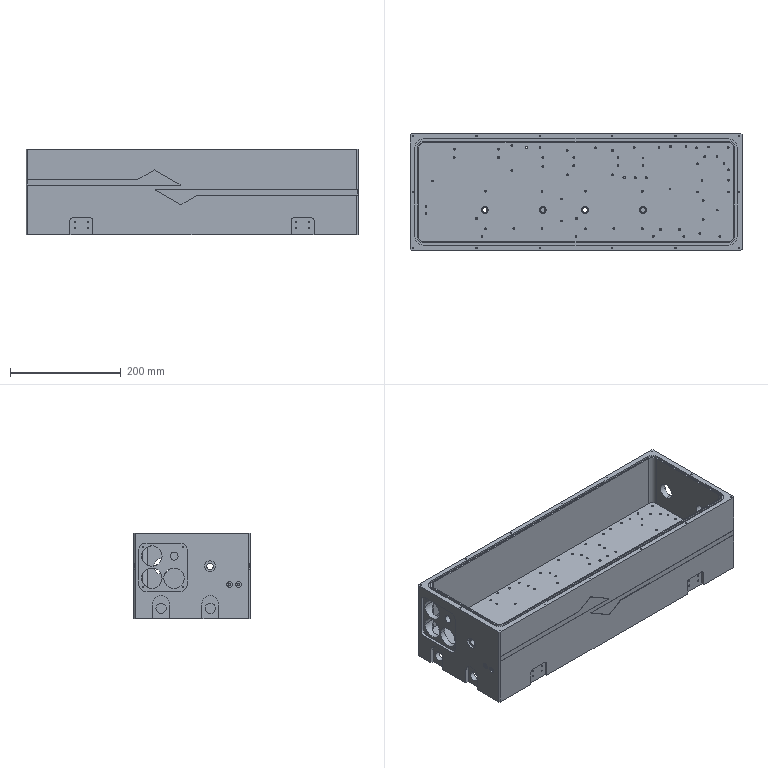Part | SolidWorks | features ICE 64, Fillet 20, 3DProfileFeature 18, HoleWzd 18, MoveFace 7, Chamfer 2, CirPattern 2, Cut 2, Extrusion 1, LPattern 1, MirrorPattern 1 | 2 solids | 912 faces | box 600 x 210 x 155 mm | volume 5602936 mm3 | cylinder 471 | cone 248 | plane 193 | commonest cylinder face diameters 3.3 x150 2.5 x96 10 x30 20 x21 24 x17 8 x16